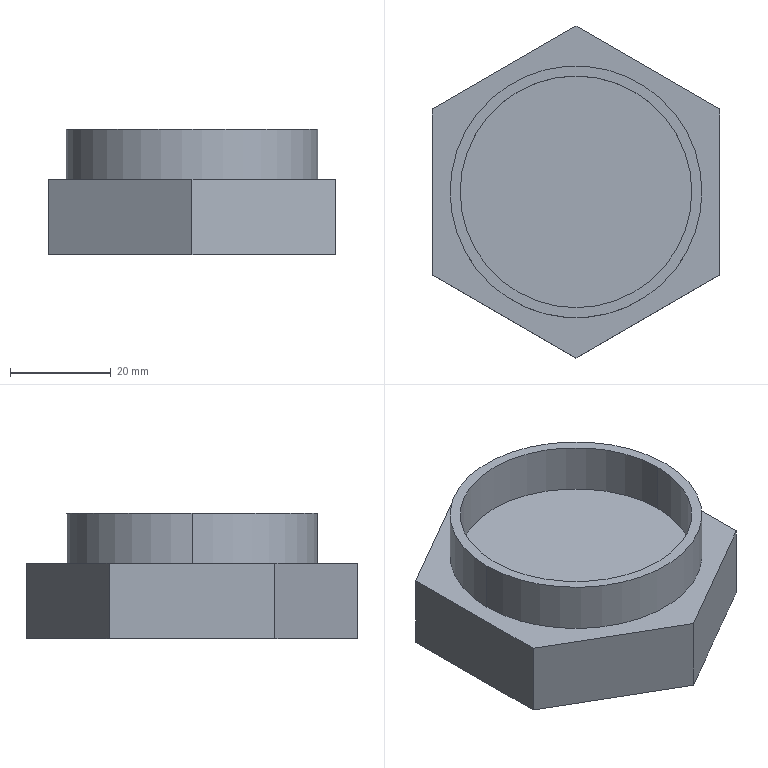Part | SolidWorks | features Extrusion 1, ICE 1 | 1 solid | 14 faces | box 57.073 x 65.902 x 25 mm | volume 45330 mm3 | plane 10 | cylinder 4 | commonest cylinder face diameters 46 x2 50 x2
STEP:
#1=CARTESIAN_POINT('',(-23.,0.,10.));
#2=VERTEX_POINT('',#1);
#3=CARTESIAN_POINT('',(23.,0.,10.));
#4=VERTEX_POINT('',#3);
#5=CARTESIAN_POINT('',(0.,0.,10.));
#6=DIRECTION('',(0.,0.,1.));
#7=DIRECTION('',(1.,0.,0.));
#8=AXIS2_PLACEMENT_3D('',#5,#6,#7);
#9=CIRCLE('',#8,23.);
#10=EDGE_CURVE('',#2,#4,#9,.T.);
#11=ORIENTED_EDGE('',*,*,#10,.T.);
#12=CARTESIAN_POINT('',(23.,0.,0.));
#13=VERTEX_POINT('',#12);
#14=CARTESIAN_POINT('',(23.,0.,10.));
#15=DIRECTION('',(0.,0.,-1.));
#16=VECTOR('',#15,1000.);
#17=LINE('',#14,#16);
#18=EDGE_CURVE('',#4,#13,#17,.T.);
#19=ORIENTED_EDGE('',*,*,#18,.T.);
#20=CARTESIAN_POINT('',(-23.,0.,0.));
#21=VERTEX_POINT('',#20);
#22=CARTESIAN_POINT('',(0.,0.,0.));
#23=DIRECTION('',(0.,0.,1.));
#24=DIRECTION('',(1.,0.,0.));
#25=AXIS2_PLACEMENT_3D('',#22,#23,#24);
#26=CIRCLE('',#25,23.);
#27=EDGE_CURVE('',#21,#13,#26,.T.);
#28=ORIENTED_EDGE('',*,*,#27,.F.);
#29=CARTESIAN_POINT('',(-23.,0.,10.));
#30=DIRECTION('',(0.,0.,-1.));
#31=VECTOR('',#30,1000.);
#32=LINE('',#29,#31);
#33=EDGE_CURVE('',#2,#21,#32,.T.);
#34=ORIENTED_EDGE('',*,*,#33,.F.);
#35=EDGE_LOOP('',(#11,#19,#28,#34));
#36=FACE_OUTER_BOUND('',#35,.T.);
#37=CARTESIAN_POINT('',(0.,0.,10.));
#38=DIRECTION('',(0.,0.,-1.));
#39=DIRECTION('',(-1.,0.,0.));
#40=AXIS2_PLACEMENT_3D('',#37,#38,#39);
#41=CYLINDRICAL_SURFACE('',#40,23.);
#42=ADVANCED_FACE('',(#36),#41,.F.);
#43=CARTESIAN_POINT('',(25.,0.,10.));
#44=VERTEX_POINT('',#43);
#45=CARTESIAN_POINT('',(-25.,0.,10.));
#46=VERTEX_POINT('',#45);
#47=CARTESIAN_POINT('',(0.,0.,10.));
#48=DIRECTION('',(0.,0.,1.));
#49=DIRECTION('',(1.,0.,0.));
#50=AXIS2_PLACEMENT_3D('',#47,#48,#49);
#51=CIRCLE('',#50,25.);
#52=EDGE_CURVE('',#44,#46,#51,.T.);
#53=ORIENTED_EDGE('',*,*,#52,.F.);
#54=CARTESIAN_POINT('',(25.,0.,0.));
#55=VERTEX_POINT('',#54);
#56=CARTESIAN_POINT('',(25.,0.,10.));
#57=DIRECTION('',(0.,0.,-1.));
#58=VECTOR('',#57,1000.);
#59=LINE('',#56,#58);
#60=EDGE_CURVE('',#44,#55,#59,.T.);
#61=ORIENTED_EDGE('',*,*,#60,.T.);
#62=CARTESIAN_POINT('',(-25.,0.,0.));
#63=VERTEX_POINT('',#62);
#64=CARTESIAN_POINT('',(0.,0.,0.));
#65=DIRECTION('',(0.,0.,1.));
#66=DIRECTION('',(1.,0.,0.));
#67=AXIS2_PLACEMENT_3D('',#64,#65,#66);
#68=CIRCLE('',#67,25.);
#69=EDGE_CURVE('',#55,#63,#68,.T.);
#70=ORIENTED_EDGE('',*,*,#69,.T.);
#71=CARTESIAN_POINT('',(-25.,0.,10.));
#72=DIRECTION('',(0.,0.,-1.));
#73=VECTOR('',#72,1000.);
#74=LINE('',#71,#73);
#75=EDGE_CURVE('',#46,#63,#74,.T.);
#76=ORIENTED_EDGE('',*,*,#75,.F.);
#77=EDGE_LOOP('',(#53,#61,#70,#76));
#78=FACE_OUTER_BOUND('',#77,.T.);
#79=CARTESIAN_POINT('',(0.,0.,10.));
#80=DIRECTION('',(0.,0.,-1.));
#81=DIRECTION('',(-1.,0.,0.));
#82=AXIS2_PLACEMENT_3D('',#79,#80,#81);
#83=CYLINDRICAL_SURFACE('',#82,25.);
#84=ADVANCED_FACE('',(#78),#83,.T.);
#85=CARTESIAN_POINT('',(0.,0.,10.));
#86=DIRECTION('',(0.,0.,1.));
#87=DIRECTION('',(1.,0.,0.));
#88=AXIS2_PLACEMENT_3D('',#85,#86,#87);
#89=CIRCLE('',#88,25.);
#90=EDGE_CURVE('',#46,#44,#89,.T.);
#91=ORIENTED_EDGE('',*,*,#90,.T.);
#92=ORIENTED_EDGE('',*,*,#52,.T.);
#93=EDGE_LOOP('',(#91,#92));
#94=FACE_OUTER_BOUND('',#93,.T.);
#95=ORIENTED_EDGE('',*,*,#10,.F.);
#96=CARTESIAN_POINT('',(0.,0.,10.));
#97=DIRECTION('',(0.,0.,1.));
#98=DIRECTION('',(1.,0.,0.));
#99=AXIS2_PLACEMENT_3D('',#96,#97,#98);
#100=CIRCLE('',#99,23.);
#101=EDGE_CURVE('',#4,#2,#100,.T.);
#102=ORIENTED_EDGE('',*,*,#101,.F.);
#103=EDGE_LOOP('',(#95,#102));
#104=FACE_BOUND('',#103,.T.);
#105=CARTESIAN_POINT('',(0.,0.,10.));
#106=DIRECTION('',(0.,0.,1.));
#107=DIRECTION('',(1.,0.,0.));
#108=AXIS2_PLACEMENT_3D('',#105,#106,#107);
#109=PLANE('',#108);
#110=ADVANCED_FACE('',(#94,#104),#109,.T.);
#111=ORIENTED_EDGE('',*,*,#60,.F.);
#112=ORIENTED_EDGE('',*,*,#90,.F.);
#113=ORIENTED_EDGE('',*,*,#75,.T.);
#114=CARTESIAN_POINT('',(0.,0.,0.));
#115=DIRECTION('',(0.,0.,1.));
#116=DIRECTION('',(1.,0.,0.));
#117=AXIS2_PLACEMENT_3D('',#114,#115,#116);
#118=CIRCLE('',#117,25.);
#119=EDGE_CURVE('',#63,#55,#118,.T.);
#120=ORIENTED_EDGE('',*,*,#119,.T.);
#121=EDGE_LOOP('',(#111,#112,#113,#120));
#122=FACE_OUTER_BOUND('',#121,.T.);
#123=CARTESIAN_POINT('',(0.,0.,10.));
#124=DIRECTION('',(0.,0.,-1.));
#125=DIRECTION('',(-1.,0.,0.));
#126=AXIS2_PLACEMENT_3D('',#123,#124,#125);
#127=CYLINDRICAL_SURFACE('',#126,25.);
#128=ADVANCED_FACE('',(#122),#127,.T.);
#129=ORIENTED_EDGE('',*,*,#18,.F.);
#130=ORIENTED_EDGE('',*,*,#101,.T.);
#131=ORIENTED_EDGE('',*,*,#33,.T.);
#132=CARTESIAN_POINT('',(0.,0.,0.));
#133=DIRECTION('',(0.,0.,1.));
#134=DIRECTION('',(1.,0.,0.));
#135=AXIS2_PLACEMENT_3D('',#132,#133,#134);
#136=CIRCLE('',#135,23.);
#137=EDGE_CURVE('',#13,#21,#136,.T.);
#138=ORIENTED_EDGE('',*,*,#137,.F.);
#139=EDGE_LOOP('',(#129,#130,#131,#138));
#140=FACE_OUTER_BOUND('',#139,.T.);
#141=CARTESIAN_POINT('',(0.,0.,10.));
#142=DIRECTION('',(0.,0.,-1.));
#143=DIRECTION('',(-1.,0.,0.));
#144=AXIS2_PLACEMENT_3D('',#141,#142,#143);
#145=CYLINDRICAL_SURFACE('',#144,23.);
#146=ADVANCED_FACE('',(#140),#145,.F.);
#147=ORIENTED_EDGE('',*,*,#27,.T.);
#148=ORIENTED_EDGE('',*,*,#137,.T.);
#149=EDGE_LOOP('',(#147,#148));
#150=FACE_OUTER_BOUND('',#149,.T.);
#151=CARTESIAN_POINT('',(0.,0.,0.));
#152=DIRECTION('',(0.,0.,-1.));
#153=DIRECTION('',(-1.,0.,0.));
#154=AXIS2_PLACEMENT_3D('',#151,#152,#153);
#155=PLANE('',#154);
#156=ADVANCED_FACE('',(#150),#155,.F.);
#157=CARTESIAN_POINT('',(-28.536,16.476,0.));
#158=VERTEX_POINT('',#157);
#159=CARTESIAN_POINT('',(0.,32.951,0.));
#160=VERTEX_POINT('',#159);
#161=CARTESIAN_POINT('',(-28.536,16.476,0.));
#162=DIRECTION('',(0.866,0.5,0.));
#163=VECTOR('',#162,1000.);
#164=LINE('',#161,#163);
#165=EDGE_CURVE('',#158,#160,#164,.T.);
#166=ORIENTED_EDGE('',*,*,#165,.T.);
#167=CARTESIAN_POINT('',(0.,32.951,-15.));
#168=VERTEX_POINT('',#167);
#169=CARTESIAN_POINT('',(0.,32.951,-15.));
#170=DIRECTION('',(0.,0.,1.));
#171=VECTOR('',#170,1000.);
#172=LINE('',#169,#171);
#173=EDGE_CURVE('',#168,#160,#172,.T.);
#174=ORIENTED_EDGE('',*,*,#173,.F.);
#175=CARTESIAN_POINT('',(-28.536,16.476,-15.));
#176=VERTEX_POINT('',#175);
#177=CARTESIAN_POINT('',(-28.536,16.476,-15.));
#178=DIRECTION('',(0.866,0.5,0.));
#179=VECTOR('',#178,1000.);
#180=LINE('',#177,#179);
#181=EDGE_CURVE('',#176,#168,#180,.T.);
#182=ORIENTED_EDGE('',*,*,#181,.F.);
#183=CARTESIAN_POINT('',(-28.536,16.476,-15.));
#184=DIRECTION('',(0.,0.,1.));
#185=VECTOR('',#184,1000.);
#186=LINE('',#183,#185);
#187=EDGE_CURVE('',#176,#158,#186,.T.);
#188=ORIENTED_EDGE('',*,*,#187,.T.);
#189=EDGE_LOOP('',(#166,#174,#182,#188));
#190=FACE_OUTER_BOUND('',#189,.T.);
#191=CARTESIAN_POINT('',(-28.536,16.476,-15.));
#192=DIRECTION('',(0.5,-0.866,0.));
#193=DIRECTION('',(0.866,0.5,0.));
#194=AXIS2_PLACEMENT_3D('',#191,#192,#193);
#195=PLANE('',#194);
#196=ADVANCED_FACE('',(#190),#195,.F.);
#197=CARTESIAN_POINT('',(28.536,16.476,0.));
#198=VERTEX_POINT('',#197);
#199=CARTESIAN_POINT('',(0.,32.951,0.));
#200=DIRECTION('',(0.866,-0.5,0.));
#201=VECTOR('',#200,1000.);
#202=LINE('',#199,#201);
#203=EDGE_CURVE('',#160,#198,#202,.T.);
#204=ORIENTED_EDGE('',*,*,#203,.T.);
#205=CARTESIAN_POINT('',(28.536,16.476,-15.));
#206=VERTEX_POINT('',#205);
#207=CARTESIAN_POINT('',(28.536,16.476,-15.));
#208=DIRECTION('',(0.,0.,1.));
#209=VECTOR('',#208,1000.);
#210=LINE('',#207,#209);
#211=EDGE_CURVE('',#206,#198,#210,.T.);
#212=ORIENTED_EDGE('',*,*,#211,.F.);
#213=CARTESIAN_POINT('',(0.,32.951,-15.));
#214=DIRECTION('',(0.866,-0.5,0.));
#215=VECTOR('',#214,1000.);
#216=LINE('',#213,#215);
#217=EDGE_CURVE('',#168,#206,#216,.T.);
#218=ORIENTED_EDGE('',*,*,#217,.F.);
#219=ORIENTED_EDGE('',*,*,#173,.T.);
#220=EDGE_LOOP('',(#204,#212,#218,#219));
#221=FACE_OUTER_BOUND('',#220,.T.);
#222=CARTESIAN_POINT('',(0.,32.951,-15.));
#223=DIRECTION('',(-0.5,-0.866,0.));
#224=DIRECTION('',(0.866,-0.5,0.));
#225=AXIS2_PLACEMENT_3D('',#222,#223,#224);
#226=PLANE('',#225);
#227=ADVANCED_FACE('',(#221),#226,.F.);
#228=CARTESIAN_POINT('',(28.536,-16.476,0.));
#229=VERTEX_POINT('',#228);
#230=CARTESIAN_POINT('',(28.536,16.476,0.));
#231=DIRECTION('',(0.,-1.,0.));
#232=VECTOR('',#231,1000.);
#233=LINE('',#230,#232);
#234=EDGE_CURVE('',#198,#229,#233,.T.);
#235=ORIENTED_EDGE('',*,*,#234,.T.);
#236=CARTESIAN_POINT('',(28.536,-16.476,-15.));
#237=VERTEX_POINT('',#236);
#238=CARTESIAN_POINT('',(28.536,-16.476,-15.));
#239=DIRECTION('',(0.,0.,1.));
#240=VECTOR('',#239,1000.);
#241=LINE('',#238,#240);
#242=EDGE_CURVE('',#237,#229,#241,.T.);
#243=ORIENTED_EDGE('',*,*,#242,.F.);
#244=CARTESIAN_POINT('',(28.536,16.476,-15.));
#245=DIRECTION('',(0.,-1.,0.));
#246=VECTOR('',#245,1000.);
#247=LINE('',#244,#246);
#248=EDGE_CURVE('',#206,#237,#247,.T.);
#249=ORIENTED_EDGE('',*,*,#248,.F.);
#250=ORIENTED_EDGE('',*,*,#211,.T.);
#251=EDGE_LOOP('',(#235,#243,#249,#250));
#252=FACE_OUTER_BOUND('',#251,.T.);
#253=CARTESIAN_POINT('',(28.536,16.476,-15.));
#254=DIRECTION('',(-1.,0.,0.));
#255=DIRECTION('',(0.,-1.,0.));
#256=AXIS2_PLACEMENT_3D('',#253,#254,#255);
#257=PLANE('',#256);
#258=ADVANCED_FACE('',(#252),#257,.F.);
#259=CARTESIAN_POINT('',(0.,-32.951,0.));
#260=VERTEX_POINT('',#259);
#261=CARTESIAN_POINT('',(28.536,-16.476,0.));
#262=DIRECTION('',(-0.866,-0.5,0.));
#263=VECTOR('',#262,1000.);
#264=LINE('',#261,#263);
#265=EDGE_CURVE('',#229,#260,#264,.T.);
#266=ORIENTED_EDGE('',*,*,#265,.T.);
#267=CARTESIAN_POINT('',(0.,-32.951,-15.));
#268=VERTEX_POINT('',#267);
#269=CARTESIAN_POINT('',(0.,-32.951,-15.));
#270=DIRECTION('',(0.,0.,1.));
#271=VECTOR('',#270,1000.);
#272=LINE('',#269,#271);
#273=EDGE_CURVE('',#268,#260,#272,.T.);
#274=ORIENTED_EDGE('',*,*,#273,.F.);
#275=CARTESIAN_POINT('',(28.536,-16.476,-15.));
#276=DIRECTION('',(-0.866,-0.5,0.));
#277=VECTOR('',#276,1000.);
#278=LINE('',#275,#277);
#279=EDGE_CURVE('',#237,#268,#278,.T.);
#280=ORIENTED_EDGE('',*,*,#279,.F.);
#281=ORIENTED_EDGE('',*,*,#242,.T.);
#282=EDGE_LOOP('',(#266,#274,#280,#281));
#283=FACE_OUTER_BOUND('',#282,.T.);
#284=CARTESIAN_POINT('',(28.536,-16.476,-15.));
#285=DIRECTION('',(-0.5,0.866,0.));
#286=DIRECTION('',(-0.866,-0.5,0.));
#287=AXIS2_PLACEMENT_3D('',#284,#285,#286);
#288=PLANE('',#287);
#289=ADVANCED_FACE('',(#283),#288,.F.);
#290=CARTESIAN_POINT('',(-28.536,-16.476,0.));
#291=VERTEX_POINT('',#290);
#292=CARTESIAN_POINT('',(0.,-32.951,0.));
#293=DIRECTION('',(-0.866,0.5,0.));
#294=VECTOR('',#293,1000.);
#295=LINE('',#292,#294);
#296=EDGE_CURVE('',#260,#291,#295,.T.);
#297=ORIENTED_EDGE('',*,*,#296,.T.);
#298=CARTESIAN_POINT('',(-28.536,-16.476,-15.));
#299=VERTEX_POINT('',#298);
#300=CARTESIAN_POINT('',(-28.536,-16.476,-15.));
#301=DIRECTION('',(0.,0.,1.));
#302=VECTOR('',#301,1000.);
#303=LINE('',#300,#302);
#304=EDGE_CURVE('',#299,#291,#303,.T.);
#305=ORIENTED_EDGE('',*,*,#304,.F.);
#306=CARTESIAN_POINT('',(0.,-32.951,-15.));
#307=DIRECTION('',(-0.866,0.5,0.));
#308=VECTOR('',#307,1000.);
#309=LINE('',#306,#308);
#310=EDGE_CURVE('',#268,#299,#309,.T.);
#311=ORIENTED_EDGE('',*,*,#310,.F.);
#312=ORIENTED_EDGE('',*,*,#273,.T.);
#313=EDGE_LOOP('',(#297,#305,#311,#312));
#314=FACE_OUTER_BOUND('',#313,.T.);
#315=CARTESIAN_POINT('',(0.,-32.951,-15.));
#316=DIRECTION('',(0.5,0.866,0.));
#317=DIRECTION('',(-0.866,0.5,0.));
#318=AXIS2_PLACEMENT_3D('',#315,#316,#317);
#319=PLANE('',#318);
#320=ADVANCED_FACE('',(#314),#319,.F.);
#321=CARTESIAN_POINT('',(-28.536,-16.476,0.));
#322=DIRECTION('',(0.,1.,0.));
#323=VECTOR('',#322,1000.);
#324=LINE('',#321,#323);
#325=EDGE_CURVE('',#291,#158,#324,.T.);
#326=ORIENTED_EDGE('',*,*,#325,.T.);
#327=ORIENTED_EDGE('',*,*,#187,.F.);
#328=CARTESIAN_POINT('',(-28.536,-16.476,-15.));
#329=DIRECTION('',(0.,1.,0.));
#330=VECTOR('',#329,1000.);
#331=LINE('',#328,#330);
#332=EDGE_CURVE('',#299,#176,#331,.T.);
#333=ORIENTED_EDGE('',*,*,#332,.F.);
#334=ORIENTED_EDGE('',*,*,#304,.T.);
#335=EDGE_LOOP('',(#326,#327,#333,#334));
#336=FACE_OUTER_BOUND('',#335,.T.);
#337=CARTESIAN_POINT('',(-28.536,-16.476,-15.));
#338=DIRECTION('',(1.,0.,0.));
#339=DIRECTION('',(0.,1.,0.));
#340=AXIS2_PLACEMENT_3D('',#337,#338,#339);
#341=PLANE('',#340);
#342=ADVANCED_FACE('',(#336),#341,.F.);
#343=ORIENTED_EDGE('',*,*,#181,.T.);
#344=ORIENTED_EDGE('',*,*,#217,.T.);
#345=ORIENTED_EDGE('',*,*,#248,.T.);
#346=ORIENTED_EDGE('',*,*,#279,.T.);
#347=ORIENTED_EDGE('',*,*,#310,.T.);
#348=ORIENTED_EDGE('',*,*,#332,.T.);
#349=EDGE_LOOP('',(#343,#344,#345,#346,#347,#348));
#350=FACE_OUTER_BOUND('',#349,.T.);
#351=CARTESIAN_POINT('',(0.,0.,-15.));
#352=DIRECTION('',(0.,0.,-1.));
#353=DIRECTION('',(-1.,0.,0.));
#354=AXIS2_PLACEMENT_3D('',#351,#352,#353);
#355=PLANE('',#354);
#356=ADVANCED_FACE('',(#350),#355,.T.);
#357=ORIENTED_EDGE('',*,*,#119,.F.);
#358=ORIENTED_EDGE('',*,*,#69,.F.);
#359=EDGE_LOOP('',(#357,#358));
#360=FACE_BOUND('',#359,.T.);
#361=ORIENTED_EDGE('',*,*,#165,.F.);
#362=ORIENTED_EDGE('',*,*,#325,.F.);
#363=ORIENTED_EDGE('',*,*,#296,.F.);
#364=ORIENTED_EDGE('',*,*,#265,.F.);
#365=ORIENTED_EDGE('',*,*,#234,.F.);
#366=ORIENTED_EDGE('',*,*,#203,.F.);
#367=EDGE_LOOP('',(#361,#362,#363,#364,#365,#366));
#368=FACE_OUTER_BOUND('',#367,.T.);
#369=CARTESIAN_POINT('',(0.,0.,0.));
#370=DIRECTION('',(0.,0.,-1.));
#371=DIRECTION('',(-1.,0.,0.));
#372=AXIS2_PLACEMENT_3D('',#369,#370,#371);
#373=PLANE('',#372);
#374=ADVANCED_FACE('',(#360,#368),#373,.F.);
#375=CLOSED_SHELL('',(#42,#84,#110,#128,#146,#156,#196,#227,#258,#289,#320,#342,#356,#374));
#376=MANIFOLD_SOLID_BREP('',#375);
#377=CARTESIAN_POINT('',(0.,0.,0.));
#378=DIRECTION('',(0.,0.,1.));
#379=DIRECTION('',(1.,0.,0.));
#380=AXIS2_PLACEMENT_3D('',#377,#378,#379);
#381=(LENGTH_UNIT()NAMED_UNIT(*)SI_UNIT(.MILLI.,.METRE.));
#382=UNCERTAINTY_MEASURE_WITH_UNIT(LENGTH_MEASURE(0.00001),#381,'','');
#383=(NAMED_UNIT(*)PLANE_ANGLE_UNIT()SI_UNIT($,.RADIAN.));
#384=(NAMED_UNIT(*)SI_UNIT($,.STERADIAN.)SOLID_ANGLE_UNIT());
#385=(GEOMETRIC_REPRESENTATION_CONTEXT(3)GLOBAL_UNCERTAINTY_ASSIGNED_CONTEXT((#382))GLOBAL_UNIT_ASSIGNED_CONTEXT((#381,#383,#384))REPRESENTATION_CONTEXT('',''));
#386=ADVANCED_BREP_SHAPE_REPRESENTATION('',(#376,#380),#385);